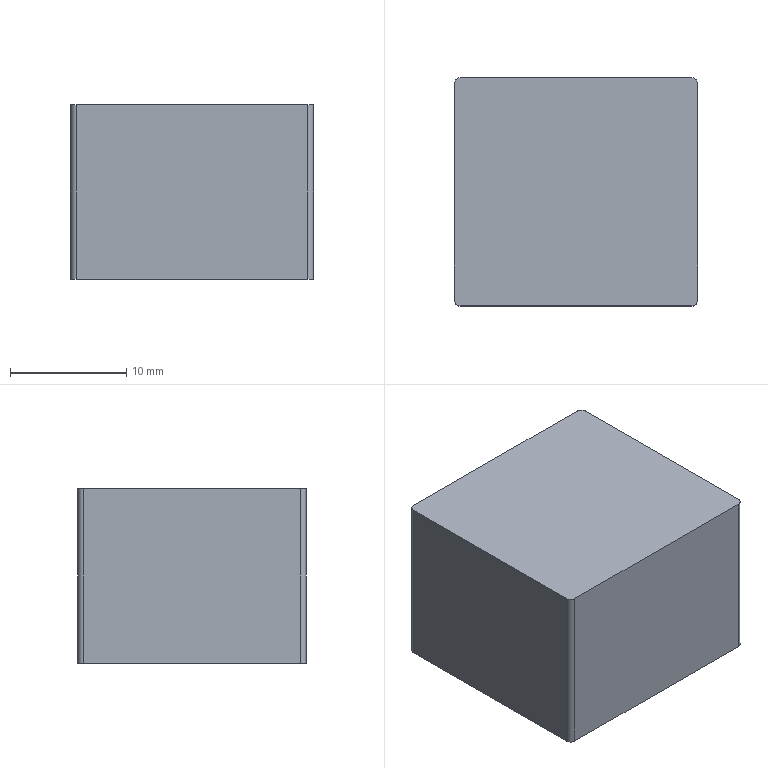Part | NX | features BREP 1 | 1 solid | 10 faces | box 20.899 x 19.607 x 15 mm | volume 6143 mm3 | plane 6 | cylinder 4 | commonest cylinder face diameters 1 x4
STEP:
#1=CARTESIAN_POINT('',(-9.95,9.804,-25.6));
#2=VERTEX_POINT('',#1);
#3=CARTESIAN_POINT('',(-10.45,9.304,-25.6));
#4=VERTEX_POINT('',#3);
#5=CARTESIAN_POINT('',(-9.95,9.304,-25.6));
#6=DIRECTION('',(0.,0.,1.));
#7=DIRECTION('',(1.,0.,0.));
#8=AXIS2_PLACEMENT_3D('',#5,#6,#7);
#9=CIRCLE('',#8,0.5);
#10=EDGE_CURVE('',#2,#4,#9,.T.);
#11=ORIENTED_EDGE('',*,*,#10,.F.);
#12=CARTESIAN_POINT('',(-9.95,9.804,-40.6));
#13=VERTEX_POINT('',#12);
#14=CARTESIAN_POINT('',(-9.95,9.804,-40.6));
#15=DIRECTION('',(0.,0.,1.));
#16=VECTOR('',#15,1000.);
#17=LINE('',#14,#16);
#18=EDGE_CURVE('',#13,#2,#17,.T.);
#19=ORIENTED_EDGE('',*,*,#18,.F.);
#20=CARTESIAN_POINT('',(-10.45,9.304,-40.6));
#21=VERTEX_POINT('',#20);
#22=CARTESIAN_POINT('',(-9.95,9.304,-40.6));
#23=DIRECTION('',(0.,0.,1.));
#24=DIRECTION('',(1.,0.,0.));
#25=AXIS2_PLACEMENT_3D('',#22,#23,#24);
#26=CIRCLE('',#25,0.5);
#27=EDGE_CURVE('',#13,#21,#26,.T.);
#28=ORIENTED_EDGE('',*,*,#27,.T.);
#29=CARTESIAN_POINT('',(-10.45,9.304,-40.6));
#30=DIRECTION('',(0.,0.,1.));
#31=VECTOR('',#30,1000.);
#32=LINE('',#29,#31);
#33=EDGE_CURVE('',#21,#4,#32,.T.);
#34=ORIENTED_EDGE('',*,*,#33,.T.);
#35=EDGE_LOOP('',(#11,#19,#28,#34));
#36=FACE_BOUND('',#35,.T.);
#37=CARTESIAN_POINT('',(-9.95,9.304,-40.6));
#38=DIRECTION('',(0.,0.,1.));
#39=DIRECTION('',(-1.,0.,0.));
#40=AXIS2_PLACEMENT_3D('',#37,#38,#39);
#41=CYLINDRICAL_SURFACE('',#40,0.5);
#42=ADVANCED_FACE('',(#36),#41,.T.);
#43=CARTESIAN_POINT('',(-10.45,-9.304,-25.6));
#44=VERTEX_POINT('',#43);
#45=CARTESIAN_POINT('',(-10.45,-9.304,-25.6));
#46=DIRECTION('',(0.,1.,0.));
#47=VECTOR('',#46,1000.);
#48=LINE('',#45,#47);
#49=EDGE_CURVE('',#44,#4,#48,.T.);
#50=ORIENTED_EDGE('',*,*,#49,.T.);
#51=ORIENTED_EDGE('',*,*,#33,.F.);
#52=CARTESIAN_POINT('',(-10.45,-9.304,-40.6));
#53=VERTEX_POINT('',#52);
#54=CARTESIAN_POINT('',(-10.45,-9.304,-40.6));
#55=DIRECTION('',(0.,1.,0.));
#56=VECTOR('',#55,1000.);
#57=LINE('',#54,#56);
#58=EDGE_CURVE('',#53,#21,#57,.T.);
#59=ORIENTED_EDGE('',*,*,#58,.F.);
#60=CARTESIAN_POINT('',(-10.45,-9.304,-40.6));
#61=DIRECTION('',(0.,0.,1.));
#62=VECTOR('',#61,1000.);
#63=LINE('',#60,#62);
#64=EDGE_CURVE('',#53,#44,#63,.T.);
#65=ORIENTED_EDGE('',*,*,#64,.T.);
#66=EDGE_LOOP('',(#50,#51,#59,#65));
#67=FACE_BOUND('',#66,.T.);
#68=CARTESIAN_POINT('',(-10.45,-9.304,-40.6));
#69=DIRECTION('',(1.,0.,0.));
#70=DIRECTION('',(0.,-1.,0.));
#71=AXIS2_PLACEMENT_3D('',#68,#69,#70);
#72=PLANE('',#71);
#73=ADVANCED_FACE('',(#67),#72,.F.);
#74=CARTESIAN_POINT('',(-9.95,-9.804,-25.6));
#75=VERTEX_POINT('',#74);
#76=CARTESIAN_POINT('',(-9.95,-9.304,-25.6));
#77=DIRECTION('',(0.,0.,1.));
#78=DIRECTION('',(1.,0.,0.));
#79=AXIS2_PLACEMENT_3D('',#76,#77,#78);
#80=CIRCLE('',#79,0.5);
#81=EDGE_CURVE('',#44,#75,#80,.T.);
#82=ORIENTED_EDGE('',*,*,#81,.F.);
#83=ORIENTED_EDGE('',*,*,#64,.F.);
#84=CARTESIAN_POINT('',(-9.95,-9.804,-40.6));
#85=VERTEX_POINT('',#84);
#86=CARTESIAN_POINT('',(-9.95,-9.304,-40.6));
#87=DIRECTION('',(0.,0.,1.));
#88=DIRECTION('',(1.,0.,0.));
#89=AXIS2_PLACEMENT_3D('',#86,#87,#88);
#90=CIRCLE('',#89,0.5);
#91=EDGE_CURVE('',#53,#85,#90,.T.);
#92=ORIENTED_EDGE('',*,*,#91,.T.);
#93=CARTESIAN_POINT('',(-9.95,-9.804,-40.6));
#94=DIRECTION('',(0.,0.,1.));
#95=VECTOR('',#94,1000.);
#96=LINE('',#93,#95);
#97=EDGE_CURVE('',#85,#75,#96,.T.);
#98=ORIENTED_EDGE('',*,*,#97,.T.);
#99=EDGE_LOOP('',(#82,#83,#92,#98));
#100=FACE_BOUND('',#99,.T.);
#101=CARTESIAN_POINT('',(-9.95,-9.304,-40.6));
#102=DIRECTION('',(0.,0.,1.));
#103=DIRECTION('',(-1.,0.,0.));
#104=AXIS2_PLACEMENT_3D('',#101,#102,#103);
#105=CYLINDRICAL_SURFACE('',#104,0.5);
#106=ADVANCED_FACE('',(#100),#105,.T.);
#107=CARTESIAN_POINT('',(9.95,-9.804,-25.6));
#108=VERTEX_POINT('',#107);
#109=CARTESIAN_POINT('',(9.95,-9.804,-25.6));
#110=DIRECTION('',(-1.,0.,0.));
#111=VECTOR('',#110,1000.);
#112=LINE('',#109,#111);
#113=EDGE_CURVE('',#108,#75,#112,.T.);
#114=ORIENTED_EDGE('',*,*,#113,.T.);
#115=ORIENTED_EDGE('',*,*,#97,.F.);
#116=CARTESIAN_POINT('',(9.95,-9.804,-40.6));
#117=VERTEX_POINT('',#116);
#118=CARTESIAN_POINT('',(9.95,-9.804,-40.6));
#119=DIRECTION('',(-1.,0.,0.));
#120=VECTOR('',#119,1000.);
#121=LINE('',#118,#120);
#122=EDGE_CURVE('',#117,#85,#121,.T.);
#123=ORIENTED_EDGE('',*,*,#122,.F.);
#124=CARTESIAN_POINT('',(9.95,-9.804,-40.6));
#125=DIRECTION('',(0.,0.,1.));
#126=VECTOR('',#125,1000.);
#127=LINE('',#124,#126);
#128=EDGE_CURVE('',#117,#108,#127,.T.);
#129=ORIENTED_EDGE('',*,*,#128,.T.);
#130=EDGE_LOOP('',(#114,#115,#123,#129));
#131=FACE_BOUND('',#130,.T.);
#132=CARTESIAN_POINT('',(9.95,-9.804,-40.6));
#133=DIRECTION('',(0.,1.,0.));
#134=DIRECTION('',(1.,0.,0.));
#135=AXIS2_PLACEMENT_3D('',#132,#133,#134);
#136=PLANE('',#135);
#137=ADVANCED_FACE('',(#131),#136,.F.);
#138=CARTESIAN_POINT('',(10.45,-9.304,-25.6));
#139=VERTEX_POINT('',#138);
#140=CARTESIAN_POINT('',(9.95,-9.304,-25.6));
#141=DIRECTION('',(0.,0.,1.));
#142=DIRECTION('',(1.,0.,0.));
#143=AXIS2_PLACEMENT_3D('',#140,#141,#142);
#144=CIRCLE('',#143,0.5);
#145=EDGE_CURVE('',#108,#139,#144,.T.);
#146=ORIENTED_EDGE('',*,*,#145,.F.);
#147=ORIENTED_EDGE('',*,*,#128,.F.);
#148=CARTESIAN_POINT('',(10.45,-9.304,-40.6));
#149=VERTEX_POINT('',#148);
#150=CARTESIAN_POINT('',(9.95,-9.304,-40.6));
#151=DIRECTION('',(0.,0.,1.));
#152=DIRECTION('',(1.,0.,0.));
#153=AXIS2_PLACEMENT_3D('',#150,#151,#152);
#154=CIRCLE('',#153,0.5);
#155=EDGE_CURVE('',#117,#149,#154,.T.);
#156=ORIENTED_EDGE('',*,*,#155,.T.);
#157=CARTESIAN_POINT('',(10.45,-9.304,-40.6));
#158=DIRECTION('',(0.,0.,1.));
#159=VECTOR('',#158,1000.);
#160=LINE('',#157,#159);
#161=EDGE_CURVE('',#149,#139,#160,.T.);
#162=ORIENTED_EDGE('',*,*,#161,.T.);
#163=EDGE_LOOP('',(#146,#147,#156,#162));
#164=FACE_BOUND('',#163,.T.);
#165=CARTESIAN_POINT('',(9.95,-9.304,-40.6));
#166=DIRECTION('',(0.,0.,1.));
#167=DIRECTION('',(-1.,0.,0.));
#168=AXIS2_PLACEMENT_3D('',#165,#166,#167);
#169=CYLINDRICAL_SURFACE('',#168,0.5);
#170=ADVANCED_FACE('',(#164),#169,.T.);
#171=CARTESIAN_POINT('',(10.45,9.304,-25.6));
#172=VERTEX_POINT('',#171);
#173=CARTESIAN_POINT('',(10.45,9.304,-25.6));
#174=DIRECTION('',(0.,-1.,0.));
#175=VECTOR('',#174,1000.);
#176=LINE('',#173,#175);
#177=EDGE_CURVE('',#172,#139,#176,.T.);
#178=ORIENTED_EDGE('',*,*,#177,.T.);
#179=ORIENTED_EDGE('',*,*,#161,.F.);
#180=CARTESIAN_POINT('',(10.45,9.304,-40.6));
#181=VERTEX_POINT('',#180);
#182=CARTESIAN_POINT('',(10.45,9.304,-40.6));
#183=DIRECTION('',(0.,-1.,0.));
#184=VECTOR('',#183,1000.);
#185=LINE('',#182,#184);
#186=EDGE_CURVE('',#181,#149,#185,.T.);
#187=ORIENTED_EDGE('',*,*,#186,.F.);
#188=CARTESIAN_POINT('',(10.45,9.304,-40.6));
#189=DIRECTION('',(0.,0.,1.));
#190=VECTOR('',#189,1000.);
#191=LINE('',#188,#190);
#192=EDGE_CURVE('',#181,#172,#191,.T.);
#193=ORIENTED_EDGE('',*,*,#192,.T.);
#194=EDGE_LOOP('',(#178,#179,#187,#193));
#195=FACE_BOUND('',#194,.T.);
#196=CARTESIAN_POINT('',(10.45,9.304,-40.6));
#197=DIRECTION('',(-1.,0.,0.));
#198=DIRECTION('',(0.,1.,0.));
#199=AXIS2_PLACEMENT_3D('',#196,#197,#198);
#200=PLANE('',#199);
#201=ADVANCED_FACE('',(#195),#200,.F.);
#202=CARTESIAN_POINT('',(9.95,9.804,-25.6));
#203=VERTEX_POINT('',#202);
#204=CARTESIAN_POINT('',(9.95,9.304,-25.6));
#205=DIRECTION('',(0.,0.,1.));
#206=DIRECTION('',(1.,0.,0.));
#207=AXIS2_PLACEMENT_3D('',#204,#205,#206);
#208=CIRCLE('',#207,0.5);
#209=EDGE_CURVE('',#172,#203,#208,.T.);
#210=ORIENTED_EDGE('',*,*,#209,.F.);
#211=ORIENTED_EDGE('',*,*,#192,.F.);
#212=CARTESIAN_POINT('',(9.95,9.804,-40.6));
#213=VERTEX_POINT('',#212);
#214=CARTESIAN_POINT('',(9.95,9.304,-40.6));
#215=DIRECTION('',(0.,0.,1.));
#216=DIRECTION('',(1.,0.,0.));
#217=AXIS2_PLACEMENT_3D('',#214,#215,#216);
#218=CIRCLE('',#217,0.5);
#219=EDGE_CURVE('',#181,#213,#218,.T.);
#220=ORIENTED_EDGE('',*,*,#219,.T.);
#221=CARTESIAN_POINT('',(9.95,9.804,-40.6));
#222=DIRECTION('',(0.,0.,1.));
#223=VECTOR('',#222,1000.);
#224=LINE('',#221,#223);
#225=EDGE_CURVE('',#213,#203,#224,.T.);
#226=ORIENTED_EDGE('',*,*,#225,.T.);
#227=EDGE_LOOP('',(#210,#211,#220,#226));
#228=FACE_BOUND('',#227,.T.);
#229=CARTESIAN_POINT('',(9.95,9.304,-40.6));
#230=DIRECTION('',(0.,0.,1.));
#231=DIRECTION('',(-1.,0.,0.));
#232=AXIS2_PLACEMENT_3D('',#229,#230,#231);
#233=CYLINDRICAL_SURFACE('',#232,0.5);
#234=ADVANCED_FACE('',(#228),#233,.T.);
#235=CARTESIAN_POINT('',(-9.95,9.804,-25.6));
#236=DIRECTION('',(1.,0.,0.));
#237=VECTOR('',#236,1000.);
#238=LINE('',#235,#237);
#239=EDGE_CURVE('',#2,#203,#238,.T.);
#240=ORIENTED_EDGE('',*,*,#239,.T.);
#241=ORIENTED_EDGE('',*,*,#225,.F.);
#242=CARTESIAN_POINT('',(-9.95,9.804,-40.6));
#243=DIRECTION('',(1.,0.,0.));
#244=VECTOR('',#243,1000.);
#245=LINE('',#242,#244);
#246=EDGE_CURVE('',#13,#213,#245,.T.);
#247=ORIENTED_EDGE('',*,*,#246,.F.);
#248=ORIENTED_EDGE('',*,*,#18,.T.);
#249=EDGE_LOOP('',(#240,#241,#247,#248));
#250=FACE_BOUND('',#249,.T.);
#251=CARTESIAN_POINT('',(-9.95,9.804,-40.6));
#252=DIRECTION('',(0.,-1.,0.));
#253=DIRECTION('',(0.,0.,1.));
#254=AXIS2_PLACEMENT_3D('',#251,#252,#253);
#255=PLANE('',#254);
#256=ADVANCED_FACE('',(#250),#255,.F.);
#257=ORIENTED_EDGE('',*,*,#27,.F.);
#258=ORIENTED_EDGE('',*,*,#246,.T.);
#259=ORIENTED_EDGE('',*,*,#219,.F.);
#260=ORIENTED_EDGE('',*,*,#186,.T.);
#261=ORIENTED_EDGE('',*,*,#155,.F.);
#262=ORIENTED_EDGE('',*,*,#122,.T.);
#263=ORIENTED_EDGE('',*,*,#91,.F.);
#264=ORIENTED_EDGE('',*,*,#58,.T.);
#265=EDGE_LOOP('',(#257,#258,#259,#260,#261,#262,#263,#264));
#266=FACE_BOUND('',#265,.T.);
#267=CARTESIAN_POINT('',(-9.95,9.304,-40.6));
#268=DIRECTION('',(0.,0.,1.));
#269=DIRECTION('',(-1.,0.,0.));
#270=AXIS2_PLACEMENT_3D('',#267,#268,#269);
#271=PLANE('',#270);
#272=ADVANCED_FACE('',(#266),#271,.F.);
#273=ORIENTED_EDGE('',*,*,#10,.T.);
#274=ORIENTED_EDGE('',*,*,#49,.F.);
#275=ORIENTED_EDGE('',*,*,#81,.T.);
#276=ORIENTED_EDGE('',*,*,#113,.F.);
#277=ORIENTED_EDGE('',*,*,#145,.T.);
#278=ORIENTED_EDGE('',*,*,#177,.F.);
#279=ORIENTED_EDGE('',*,*,#209,.T.);
#280=ORIENTED_EDGE('',*,*,#239,.F.);
#281=EDGE_LOOP('',(#273,#274,#275,#276,#277,#278,#279,#280));
#282=FACE_BOUND('',#281,.T.);
#283=CARTESIAN_POINT('',(-9.95,9.304,-25.6));
#284=DIRECTION('',(0.,0.,1.));
#285=DIRECTION('',(-1.,0.,0.));
#286=AXIS2_PLACEMENT_3D('',#283,#284,#285);
#287=PLANE('',#286);
#288=ADVANCED_FACE('',(#282),#287,.T.);
#289=CLOSED_SHELL('',(#42,#73,#106,#137,#170,#201,#234,#256,#272,#288));
#290=MANIFOLD_SOLID_BREP('',#289);
#291=(LENGTH_UNIT()NAMED_UNIT(*)SI_UNIT(.MILLI.,.METRE.));
#292=UNCERTAINTY_MEASURE_WITH_UNIT(LENGTH_MEASURE(0.00001),#291,'','');
#293=(NAMED_UNIT(*)PLANE_ANGLE_UNIT()SI_UNIT($,.RADIAN.));
#294=(NAMED_UNIT(*)SI_UNIT($,.STERADIAN.)SOLID_ANGLE_UNIT());
#295=(GEOMETRIC_REPRESENTATION_CONTEXT(3)GLOBAL_UNCERTAINTY_ASSIGNED_CONTEXT((#292))GLOBAL_UNIT_ASSIGNED_CONTEXT((#291,#293,#294))REPRESENTATION_CONTEXT('',''));
#296=ADVANCED_BREP_SHAPE_REPRESENTATION('',(#290),#295);